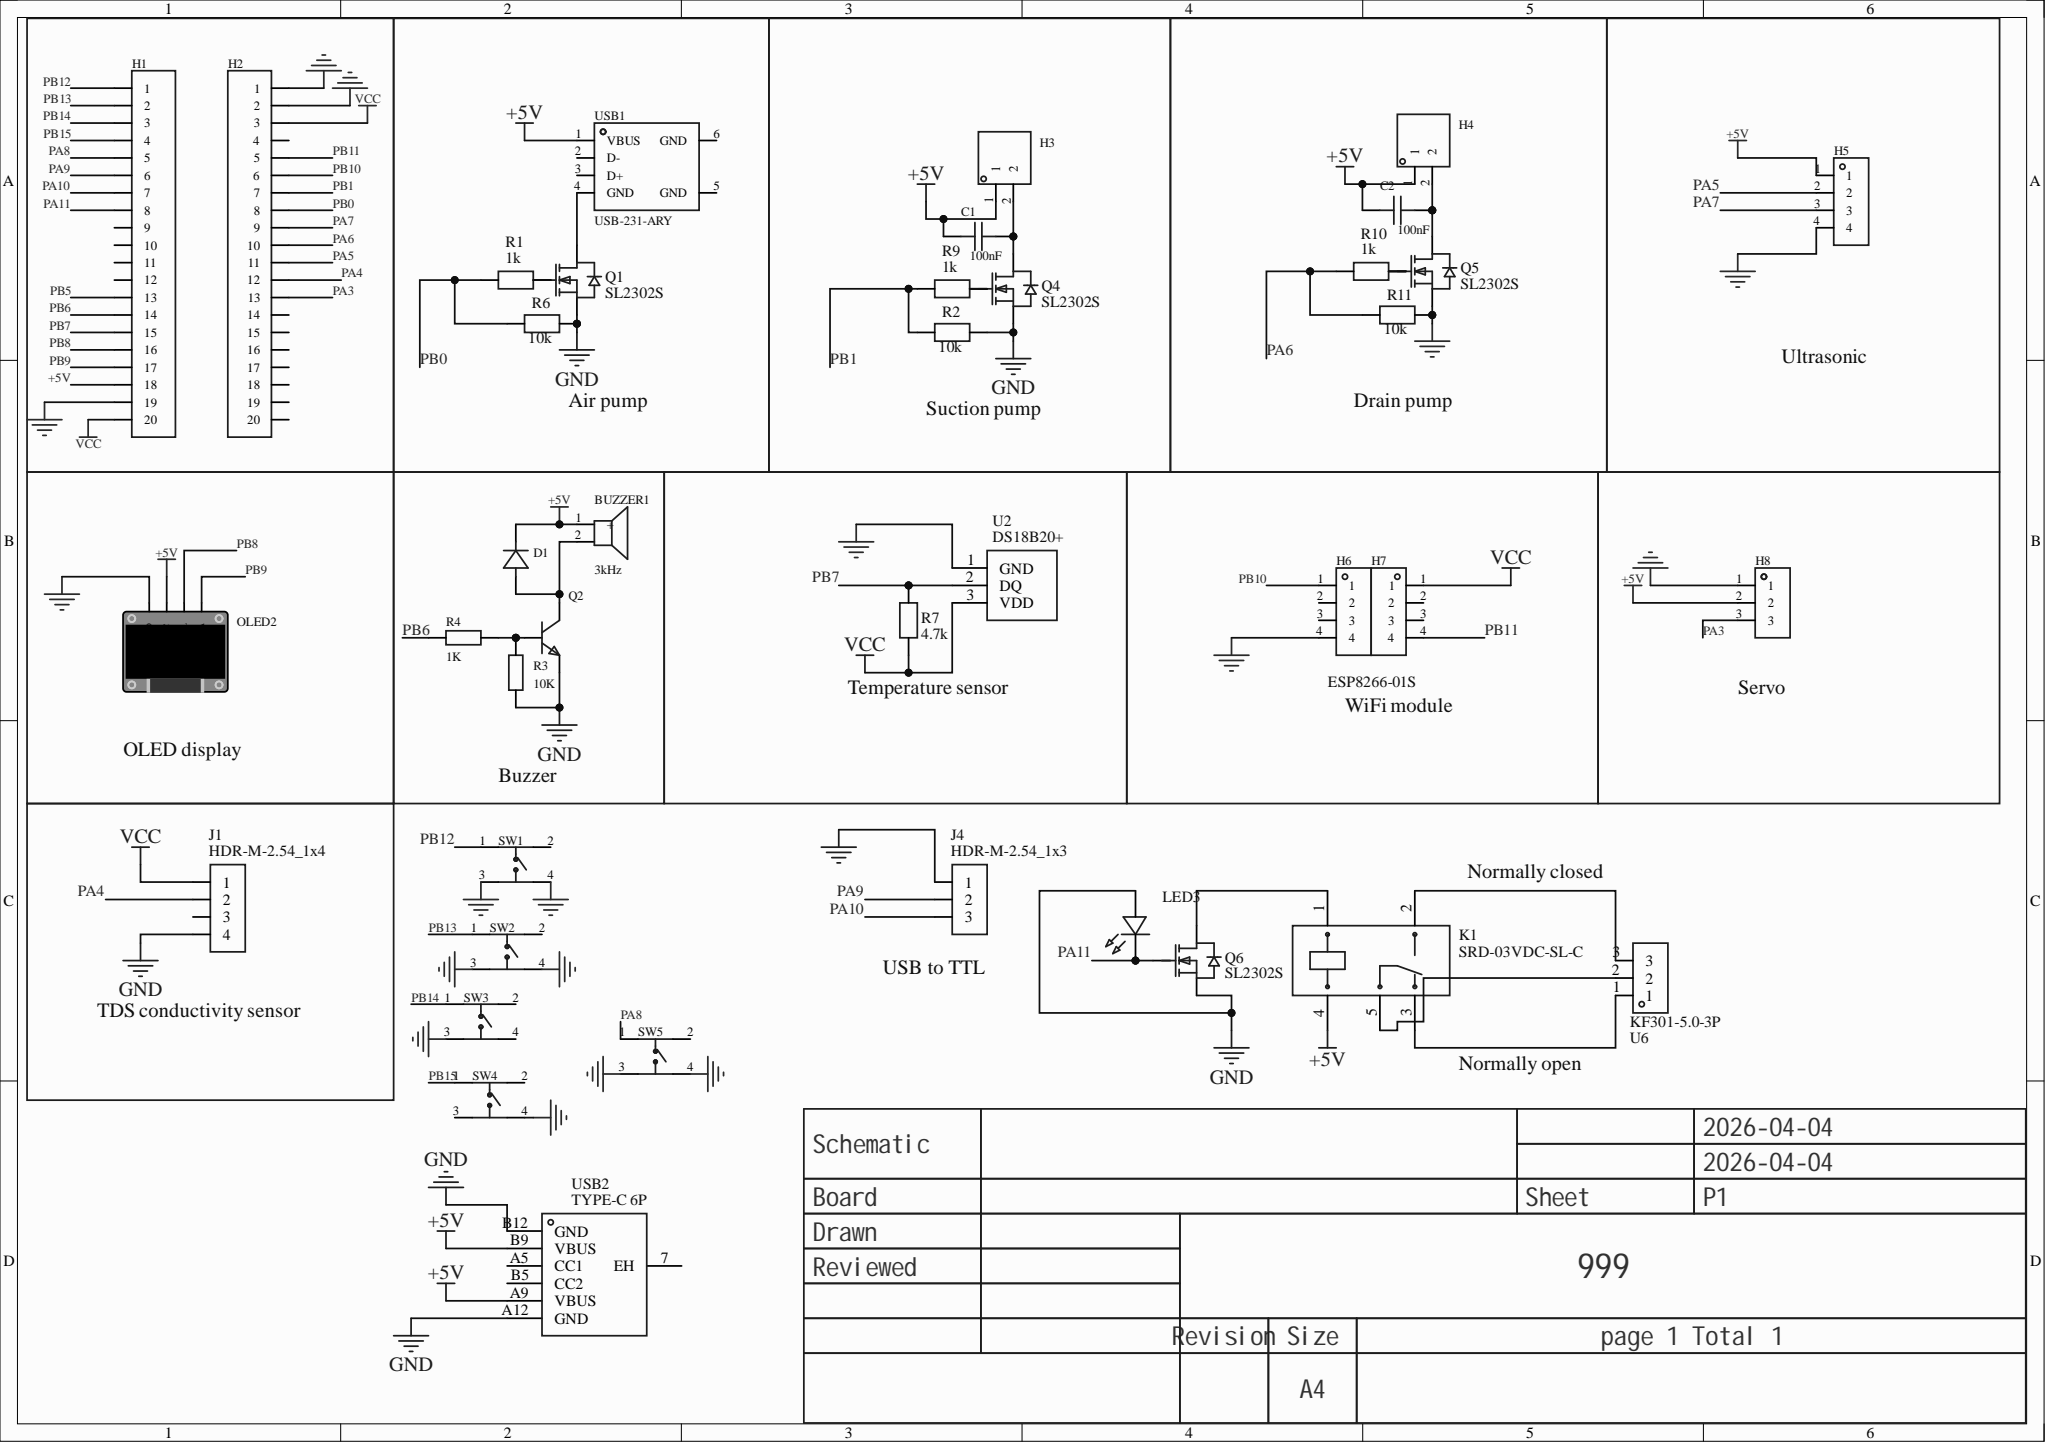Circuit board | Altium Designer | 40 parts | 36 nets
Bill of materials:
Comment,Description,Designator,Footprint,LibRef,Quantity
"3kHz","Driver type: active (built-in driver circuit); construction type: electromagnetic; rated voltage: -; frequency: 3kHz; sound pressure (SPL): 85dB;","BUZZER1","BUZ-TH_BD9.6-P5.00-D0.7-FD","HNB09A05","1"
"100nF","","C1, C2","C0805","CAP_0805","2"
"","","D1","DO_1N4007","D_1N4007A","1"
"","","H1, H2","HDR-TH_20P-P2.54-V-F","HDR-F_2.54_1x20P","2"
"","","H3, H4","HDR-TH_2P-P2.54-V-M-1","HDR-M_2.54_1x2P","2"
"","","H5, H6, H7","HDR-TH_4P-P2.54-V-M","HDR-M_2.54_1x4P","3"
"","","H8","HDR-TH_3P-P2.54-V-M","HDR-M_2.54_1x3P","1"
"HDR-M-2.54_1x4","","J1","HDR-M-2.54_1X4","HDR-M-2.54_1x4","1"
"HDR-M-2.54_1x3","","J4","HDR-M-2.54_1X3","HDR-M-2.54_1x3","1"
"SRD-03VDC-SL-C","","K1","RELAY-TH_SRD-XXVDC-XL-C","SRD-03VDC-SL-C","1"
"LED-TH-5mm_R","","LED3","LED-TH_BD5.0_RED","LED-TH-5mm_R","1"
"","","OLED2","0.96OLED_4P","0.96OLED模块_4P","1"
"SL2302S","","Q1, Q4, Q5, Q6","SOT-23_L2.9-W1.3-P1.90-LS2.4-BR","SL2302S","4"
"","","Q2","S8050_TO_92","S8050_TO_NPN","1"
"1k","","R1, R4, R9, R10","R0603","1k, Res_0603","4"
"10k","","R2, R3, R6, R11","R0603","10k, Res_0603","4"
"4.7k","","R7","R0603","10k","1"
"J1L0503110","","SW1, SW2, SW3, SW4, SW5","SW-TH_4P-L6.0-W6.0-P4.50-LS6.3","J1L0503110","5"
"DS18B20+","","U2","TO-92-3_L4.9-W3.7-P1.27-L","DS18B20+","1"
"KF301-5.0-3P","","U6","CONN-TH_3P-P5.00_KF301-5.0-3P","KF301-5.0-3P","1"
"USB-231-ARY","","USB1","USB-A-TH_USB-231-ARY","USB-231-ARY","1"
"TYPE-C 6P","","USB2","TYPE-C-SMD_TYPE-C-6P_1","TYPE-C 6P","1"
Netlist (Protel format):
[
BUZZER1
BUZ-TH_BD9.6-P5.00-D0.7-FD
3kHz



]
[
C1
C0805
100nF



]
[
C2
C0805
100nF



]
[
D1
DO_1N4007




]
[
H1
HDR-TH_20P-P2.54-V-F




]
[
H2
HDR-TH_20P-P2.54-V-F




]
[
H3
HDR-TH_2P-P2.54-V-M-1




]
[
H4
HDR-TH_2P-P2.54-V-M-1




]
[
H5
HDR-TH_4P-P2.54-V-M




]
[
H6
HDR-TH_4P-P2.54-V-M




]
[
H7
HDR-TH_4P-P2.54-V-M




]
[
H8
HDR-TH_3P-P2.54-V-M




]
[
J1
HDR-M-2.54_1X4
HDR-M-2.54_1x4



]
[
J4
HDR-M-2.54_1X3
HDR-M-2.54_1x3



]
[
K1
RELAY-TH_SRD-XXVDC-XL-C
SRD-03VDC-SL-C



]
[
LED3
LED-TH_BD5.0_RED
LED-TH-5mm_R



]
[
OLED2
0.96OLED_4P




]
[
Q1
SOT-23_L2.9-W1.3-P1.90-LS2.4-BR
SL2302S



]
[
Q2
S8050_TO_92




]
[
Q4
SOT-23_L2.9-W1.3-P1.90-LS2.4-BR
SL2302S



]
[
Q5
SOT-23_L2.9-W1.3-P1.90-LS2.4-BR
SL2302S



]
[
Q6
SOT-23_L2.9-W1.3-P1.90-LS2.4-BR
SL2302S



]
[
R1
R0603
1k



]
[
R2
R0603
10k



]
[
R3
R0603
10K



]
[
R4
R0603
1K



]
[
R6
R0603
10k



]
[
R7
R0603
4.7k



]
[
R9
R0603
1k



]
[
R10
R0603
1k



]
[
R11
R0603
10k



]
[
SW1
SW-TH_4P-L6.0-W6.0-P4.50-LS6.3
J1L0503110



]
[
SW2
SW-TH_4P-L6.0-W6.0-P4.50-LS6.3
J1L0503110



]
[
SW3
SW-TH_4P-L6.0-W6.0-P4.50-LS6.3
J1L0503110



]
[
SW4
SW-TH_4P-L6.0-W6.0-P4.50-LS6.3
J1L0503110



]
[
SW5
SW-TH_4P-L6.0-W6.0-P4.50-LS6.3
J1L0503110



]
[
U2
TO-92-3_L4.9-W3.7-P1.27-L
DS18B20+



]
[
U6
CONN-TH_3P-P5.00_KF301-5.0-3P
KF301-5.0-3P



]
[
USB1
USB-A-TH_USB-231-ARY
USB-231-ARY



]
[
USB2
TYPE-C-SMD_TYPE-C-6P_1
TYPE-C 6P



]
(
VCC
H1-20
H2-3
H7-1
J1-1
R7-2
U2-3
)
(
PB15
H1-4
SW4-1
)
(
PB14
H1-3
SW3-1
)
(
PB13
H1-2
SW2-1
)
(
PB12
H1-1
SW1-1
)
(
PB11
H2-5
H7-4
)
(
PB10
H2-6
H6-1
)
(
PB9
H1-17
OLED2-4
)
(
PB8
H1-16
OLED2-3
)
(
PB7
H1-15
R7-1
U2-2
)
(
PB6
H1-14
R4-2
)
(
PB1
H2-7
R2-1
R9-1
)
(
PB0
H2-8
R1-1
R6-1
)
(
PA11
H1-8
LED3-2
Q6-1
)
(
PA10
H1-7
J4-3
)
(
PA9
H1-6
J4-2
)
(
PA8
H1-5
SW5-1
)
(
PA7
H2-9
H5-3
)
(
PA6
H2-10
R10-1
R11-1
)
(
PA5
H2-11
H5-2
)
(
PA4
H2-12
J1-2
)
(
PA3
H2-13
H8-3
)
(
NetQ5_1
Q5-1
R10-2
)
(
NetQ4_1
Q4-1
R9-2
)
(
NetQ2_2
Q2-2
R3-2
R4-1
)
(
NetQ1_3
Q1-3
USB1-4
)
(
NetQ1_1
Q1-1
R1-2
)
(
NetK1_5
K1-5
U6-2
)
(
NetK1_3
K1-3
U6-1
)
(
NetK1_2
K1-2
U6-3
)
(
NetK1_1
K1-1
Q6-3
)
(
NetC2_2
C2-2
H4-2
Q5-3
)
(
NetC1_2
C1-2
H3-2
Q4-3
)
(
NetBUZZER1_2
BUZZER1-2
D1-2
Q2-3
)
(
GND
H1-19
H2-1
H2-2
H5-4
H6-4
H8-1
J1-4
J4-1
LED3-1
OLED2-1
Q1-2
Q2-1
Q4-2
Q5-2
Q6-2
R2-2
R3-1
R6-2
R11-2
SW1-3
SW1-4
SW2-3
SW2-4
SW3-3
SW4-4
SW5-3
SW5-4
U2-1
USB2-A12
USB2-B12
)
(
+5V
BUZZER1-1
C1-1
C2-1
D1-1
H1-18
H3-1
H4-1
H5-1
H8-2
K1-4
OLED2-2
USB1-1
USB2-A9
USB2-B9
)